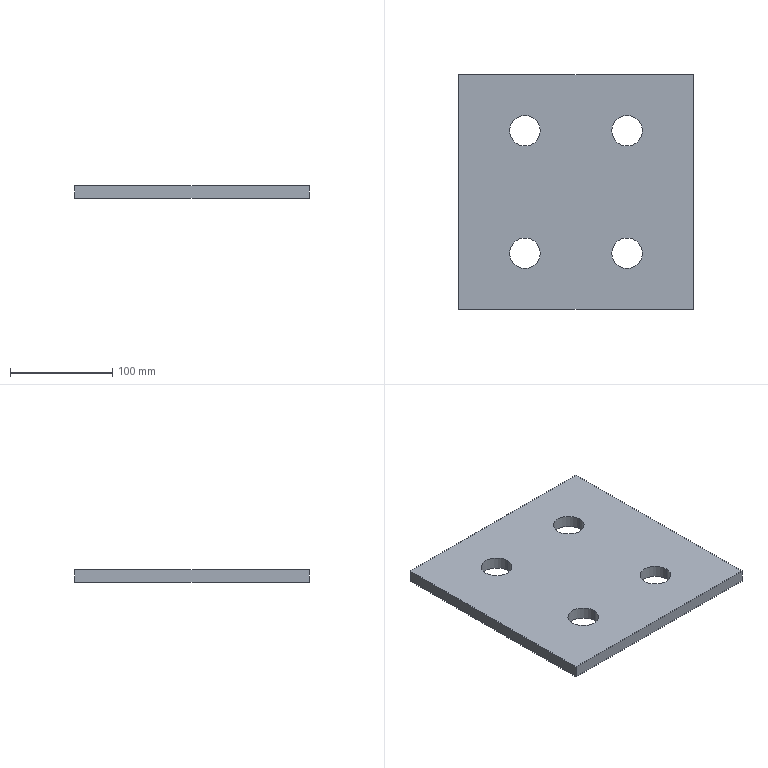Part | STEP file | Reinforcing plate 4 | 1 solid | 14 faces | box 230 x 230 x 12 mm | volume 600871 mm3 | cylinder 8 | plane 6 | commonest cylinder face diameters 30 x8
STEP:
#1=CARTESIAN_POINT('',(0.,0.,0.));
#2=DIRECTION('',(0.,0.,1.));
#3=DIRECTION('',(1.,0.,0.));
#4=AXIS2_PLACEMENT_3D('',#1,#2,#3);
#5=CARTESIAN_POINT('',(35.,-45.,12.));
#6=VERTEX_POINT('',#5);
#7=CARTESIAN_POINT('',(35.,-45.,0.));
#8=VERTEX_POINT('',#7);
#9=CARTESIAN_POINT('',(35.,-45.,12.));
#10=DIRECTION('',(0.,0.,-1.));
#11=VECTOR('',#10,1.);
#12=LINE('',#9,#11);
#13=CARTESIAN_POINT('',(50.,-45.,12.));
#14=DIRECTION('',(0.,0.,-1.));
#15=DIRECTION('',(-1.,0.,0.));
#16=AXIS2_PLACEMENT_3D('',#13,#14,#15);
#17=CYLINDRICAL_SURFACE('',#16,15.);
#18=CARTESIAN_POINT('',(6.283,0.));
#19=DIRECTION('',(0.,1.));
#20=VECTOR('',#19,1.);
#21=LINE('',#18,#20);
#22=(GEOMETRIC_REPRESENTATION_CONTEXT(2)PARAMETRIC_REPRESENTATION_CONTEXT()REPRESENTATION_CONTEXT('',''));
#23=DEFINITIONAL_REPRESENTATION('',(#21),#22);
#24=PCURVE('',#17,#23);
#25=CARTESIAN_POINT('',(50.,-45.,12.));
#26=DIRECTION('',(0.,0.,-1.));
#27=DIRECTION('',(-1.,0.,0.));
#28=AXIS2_PLACEMENT_3D('',#25,#26,#27);
#29=CYLINDRICAL_SURFACE('',#28,15.);
#30=CARTESIAN_POINT('',(0.,0.));
#31=DIRECTION('',(0.,1.));
#32=VECTOR('',#31,1.);
#33=LINE('',#30,#32);
#34=(GEOMETRIC_REPRESENTATION_CONTEXT(2)PARAMETRIC_REPRESENTATION_CONTEXT()REPRESENTATION_CONTEXT('',''));
#35=DEFINITIONAL_REPRESENTATION('',(#33),#34);
#36=PCURVE('',#29,#35);
#37=SURFACE_CURVE('',#12,(#24,#36),.PCURVE_S1.);
#38=EDGE_CURVE('',#6,#8,#37,.T.);
#39=ORIENTED_EDGE('',*,*,#38,.T.);
#40=CARTESIAN_POINT('',(65.,-45.,0.));
#41=VERTEX_POINT('',#40);
#42=CARTESIAN_POINT('',(50.,-45.,0.));
#43=DIRECTION('',(0.,0.,1.));
#44=DIRECTION('',(1.,0.,0.));
#45=AXIS2_PLACEMENT_3D('',#42,#43,#44);
#46=CIRCLE('',#45,15.);
#47=CARTESIAN_POINT('',(9.425,12.));
#48=DIRECTION('',(-1.,0.));
#49=VECTOR('',#48,1.);
#50=LINE('',#47,#49);
#51=(GEOMETRIC_REPRESENTATION_CONTEXT(2)PARAMETRIC_REPRESENTATION_CONTEXT()REPRESENTATION_CONTEXT('',''));
#52=DEFINITIONAL_REPRESENTATION('',(#50),#51);
#53=PCURVE('',#17,#52);
#54=CARTESIAN_POINT('',(115.,-100.,0.));
#55=DIRECTION('',(0.,0.,1.));
#56=DIRECTION('',(1.,0.,0.));
#57=AXIS2_PLACEMENT_3D('',#54,#55,#56);
#58=PLANE('',#57);
#59=CARTESIAN_POINT('',(-65.,55.));
#60=DIRECTION('',(1.,0.));
#61=AXIS2_PLACEMENT_2D('',#59,#60);
#62=CIRCLE('',#61,15.);
#63=(GEOMETRIC_REPRESENTATION_CONTEXT(2)PARAMETRIC_REPRESENTATION_CONTEXT()REPRESENTATION_CONTEXT('',''));
#64=DEFINITIONAL_REPRESENTATION('',(#62),#63);
#65=PCURVE('',#58,#64);
#66=SURFACE_CURVE('',#46,(#53,#65),.PCURVE_S1.);
#67=EDGE_CURVE('',#8,#41,#66,.T.);
#68=ORIENTED_EDGE('',*,*,#67,.T.);
#69=CARTESIAN_POINT('',(65.,-45.,12.));
#70=VERTEX_POINT('',#69);
#71=CARTESIAN_POINT('',(65.,-45.,12.));
#72=DIRECTION('',(0.,0.,-1.));
#73=VECTOR('',#72,1.);
#74=LINE('',#71,#73);
#75=CARTESIAN_POINT('',(3.142,0.));
#76=DIRECTION('',(0.,1.));
#77=VECTOR('',#76,1.);
#78=LINE('',#75,#77);
#79=(GEOMETRIC_REPRESENTATION_CONTEXT(2)PARAMETRIC_REPRESENTATION_CONTEXT()REPRESENTATION_CONTEXT('',''));
#80=DEFINITIONAL_REPRESENTATION('',(#78),#79);
#81=PCURVE('',#17,#80);
#82=CARTESIAN_POINT('',(3.142,0.));
#83=DIRECTION('',(0.,1.));
#84=VECTOR('',#83,1.);
#85=LINE('',#82,#84);
#86=(GEOMETRIC_REPRESENTATION_CONTEXT(2)PARAMETRIC_REPRESENTATION_CONTEXT()REPRESENTATION_CONTEXT('',''));
#87=DEFINITIONAL_REPRESENTATION('',(#85),#86);
#88=PCURVE('',#29,#87);
#89=SURFACE_CURVE('',#74,(#81,#88),.PCURVE_S1.);
#90=EDGE_CURVE('',#70,#41,#89,.T.);
#91=ORIENTED_EDGE('',*,*,#90,.F.);
#92=CARTESIAN_POINT('',(50.,-45.,12.));
#93=DIRECTION('',(0.,0.,1.));
#94=DIRECTION('',(1.,0.,0.));
#95=AXIS2_PLACEMENT_3D('',#92,#93,#94);
#96=CIRCLE('',#95,15.);
#97=CARTESIAN_POINT('',(9.425,0.));
#98=DIRECTION('',(-1.,0.));
#99=VECTOR('',#98,1.);
#100=LINE('',#97,#99);
#101=(GEOMETRIC_REPRESENTATION_CONTEXT(2)PARAMETRIC_REPRESENTATION_CONTEXT()REPRESENTATION_CONTEXT('',''));
#102=DEFINITIONAL_REPRESENTATION('',(#100),#101);
#103=PCURVE('',#17,#102);
#104=CARTESIAN_POINT('',(115.,-100.,12.));
#105=DIRECTION('',(0.,0.,1.));
#106=DIRECTION('',(1.,0.,0.));
#107=AXIS2_PLACEMENT_3D('',#104,#105,#106);
#108=PLANE('',#107);
#109=CARTESIAN_POINT('',(-65.,55.));
#110=DIRECTION('',(1.,0.));
#111=AXIS2_PLACEMENT_2D('',#109,#110);
#112=CIRCLE('',#111,15.);
#113=(GEOMETRIC_REPRESENTATION_CONTEXT(2)PARAMETRIC_REPRESENTATION_CONTEXT()REPRESENTATION_CONTEXT('',''));
#114=DEFINITIONAL_REPRESENTATION('',(#112),#113);
#115=PCURVE('',#108,#114);
#116=SURFACE_CURVE('',#96,(#103,#115),.PCURVE_S1.);
#117=EDGE_CURVE('',#6,#70,#116,.T.);
#118=ORIENTED_EDGE('',*,*,#117,.F.);
#119=EDGE_LOOP('',(#39,#68,#91,#118));
#120=FACE_BOUND('',#119,.F.);
#121=ADVANCED_FACE('',(#120),#17,.F.);
#122=CARTESIAN_POINT('',(-65.,-45.,12.));
#123=VERTEX_POINT('',#122);
#124=CARTESIAN_POINT('',(-65.,-45.,0.));
#125=VERTEX_POINT('',#124);
#126=CARTESIAN_POINT('',(-65.,-45.,12.));
#127=DIRECTION('',(0.,0.,-1.));
#128=VECTOR('',#127,1.);
#129=LINE('',#126,#128);
#130=CARTESIAN_POINT('',(-50.,-45.,12.));
#131=DIRECTION('',(0.,0.,-1.));
#132=DIRECTION('',(-1.,0.,0.));
#133=AXIS2_PLACEMENT_3D('',#130,#131,#132);
#134=CYLINDRICAL_SURFACE('',#133,15.);
#135=CARTESIAN_POINT('',(6.283,0.));
#136=DIRECTION('',(0.,1.));
#137=VECTOR('',#136,1.);
#138=LINE('',#135,#137);
#139=(GEOMETRIC_REPRESENTATION_CONTEXT(2)PARAMETRIC_REPRESENTATION_CONTEXT()REPRESENTATION_CONTEXT('',''));
#140=DEFINITIONAL_REPRESENTATION('',(#138),#139);
#141=PCURVE('',#134,#140);
#142=CARTESIAN_POINT('',(-50.,-45.,12.));
#143=DIRECTION('',(0.,0.,-1.));
#144=DIRECTION('',(-1.,0.,0.));
#145=AXIS2_PLACEMENT_3D('',#142,#143,#144);
#146=CYLINDRICAL_SURFACE('',#145,15.);
#147=CARTESIAN_POINT('',(0.,0.));
#148=DIRECTION('',(0.,1.));
#149=VECTOR('',#148,1.);
#150=LINE('',#147,#149);
#151=(GEOMETRIC_REPRESENTATION_CONTEXT(2)PARAMETRIC_REPRESENTATION_CONTEXT()REPRESENTATION_CONTEXT('',''));
#152=DEFINITIONAL_REPRESENTATION('',(#150),#151);
#153=PCURVE('',#146,#152);
#154=SURFACE_CURVE('',#129,(#141,#153),.PCURVE_S1.);
#155=EDGE_CURVE('',#123,#125,#154,.T.);
#156=ORIENTED_EDGE('',*,*,#155,.T.);
#157=CARTESIAN_POINT('',(-35.,-45.,0.));
#158=VERTEX_POINT('',#157);
#159=CARTESIAN_POINT('',(-50.,-45.,0.));
#160=DIRECTION('',(0.,0.,1.));
#161=DIRECTION('',(1.,0.,0.));
#162=AXIS2_PLACEMENT_3D('',#159,#160,#161);
#163=CIRCLE('',#162,15.);
#164=CARTESIAN_POINT('',(9.425,12.));
#165=DIRECTION('',(-1.,0.));
#166=VECTOR('',#165,1.);
#167=LINE('',#164,#166);
#168=(GEOMETRIC_REPRESENTATION_CONTEXT(2)PARAMETRIC_REPRESENTATION_CONTEXT()REPRESENTATION_CONTEXT('',''));
#169=DEFINITIONAL_REPRESENTATION('',(#167),#168);
#170=PCURVE('',#134,#169);
#171=CARTESIAN_POINT('',(-165.,55.));
#172=DIRECTION('',(1.,0.));
#173=AXIS2_PLACEMENT_2D('',#171,#172);
#174=CIRCLE('',#173,15.);
#175=(GEOMETRIC_REPRESENTATION_CONTEXT(2)PARAMETRIC_REPRESENTATION_CONTEXT()REPRESENTATION_CONTEXT('',''));
#176=DEFINITIONAL_REPRESENTATION('',(#174),#175);
#177=PCURVE('',#58,#176);
#178=SURFACE_CURVE('',#163,(#170,#177),.PCURVE_S1.);
#179=EDGE_CURVE('',#125,#158,#178,.T.);
#180=ORIENTED_EDGE('',*,*,#179,.T.);
#181=CARTESIAN_POINT('',(-35.,-45.,12.));
#182=VERTEX_POINT('',#181);
#183=CARTESIAN_POINT('',(-35.,-45.,12.));
#184=DIRECTION('',(0.,0.,-1.));
#185=VECTOR('',#184,1.);
#186=LINE('',#183,#185);
#187=CARTESIAN_POINT('',(3.142,0.));
#188=DIRECTION('',(0.,1.));
#189=VECTOR('',#188,1.);
#190=LINE('',#187,#189);
#191=(GEOMETRIC_REPRESENTATION_CONTEXT(2)PARAMETRIC_REPRESENTATION_CONTEXT()REPRESENTATION_CONTEXT('',''));
#192=DEFINITIONAL_REPRESENTATION('',(#190),#191);
#193=PCURVE('',#134,#192);
#194=CARTESIAN_POINT('',(3.142,0.));
#195=DIRECTION('',(0.,1.));
#196=VECTOR('',#195,1.);
#197=LINE('',#194,#196);
#198=(GEOMETRIC_REPRESENTATION_CONTEXT(2)PARAMETRIC_REPRESENTATION_CONTEXT()REPRESENTATION_CONTEXT('',''));
#199=DEFINITIONAL_REPRESENTATION('',(#197),#198);
#200=PCURVE('',#146,#199);
#201=SURFACE_CURVE('',#186,(#193,#200),.PCURVE_S1.);
#202=EDGE_CURVE('',#182,#158,#201,.T.);
#203=ORIENTED_EDGE('',*,*,#202,.F.);
#204=CARTESIAN_POINT('',(-50.,-45.,12.));
#205=DIRECTION('',(0.,0.,1.));
#206=DIRECTION('',(1.,0.,0.));
#207=AXIS2_PLACEMENT_3D('',#204,#205,#206);
#208=CIRCLE('',#207,15.);
#209=CARTESIAN_POINT('',(9.425,0.));
#210=DIRECTION('',(-1.,0.));
#211=VECTOR('',#210,1.);
#212=LINE('',#209,#211);
#213=(GEOMETRIC_REPRESENTATION_CONTEXT(2)PARAMETRIC_REPRESENTATION_CONTEXT()REPRESENTATION_CONTEXT('',''));
#214=DEFINITIONAL_REPRESENTATION('',(#212),#213);
#215=PCURVE('',#134,#214);
#216=CARTESIAN_POINT('',(-165.,55.));
#217=DIRECTION('',(1.,0.));
#218=AXIS2_PLACEMENT_2D('',#216,#217);
#219=CIRCLE('',#218,15.);
#220=(GEOMETRIC_REPRESENTATION_CONTEXT(2)PARAMETRIC_REPRESENTATION_CONTEXT()REPRESENTATION_CONTEXT('',''));
#221=DEFINITIONAL_REPRESENTATION('',(#219),#220);
#222=PCURVE('',#108,#221);
#223=SURFACE_CURVE('',#208,(#215,#222),.PCURVE_S1.);
#224=EDGE_CURVE('',#123,#182,#223,.T.);
#225=ORIENTED_EDGE('',*,*,#224,.F.);
#226=EDGE_LOOP('',(#156,#180,#203,#225));
#227=FACE_BOUND('',#226,.F.);
#228=ADVANCED_FACE('',(#227),#134,.F.);
#229=CARTESIAN_POINT('',(35.,75.,12.));
#230=VERTEX_POINT('',#229);
#231=CARTESIAN_POINT('',(35.,75.,0.));
#232=VERTEX_POINT('',#231);
#233=CARTESIAN_POINT('',(35.,75.,12.));
#234=DIRECTION('',(0.,0.,-1.));
#235=VECTOR('',#234,1.);
#236=LINE('',#233,#235);
#237=CARTESIAN_POINT('',(50.,75.,12.));
#238=DIRECTION('',(0.,0.,-1.));
#239=DIRECTION('',(-1.,0.,0.));
#240=AXIS2_PLACEMENT_3D('',#237,#238,#239);
#241=CYLINDRICAL_SURFACE('',#240,15.);
#242=CARTESIAN_POINT('',(6.283,0.));
#243=DIRECTION('',(0.,1.));
#244=VECTOR('',#243,1.);
#245=LINE('',#242,#244);
#246=(GEOMETRIC_REPRESENTATION_CONTEXT(2)PARAMETRIC_REPRESENTATION_CONTEXT()REPRESENTATION_CONTEXT('',''));
#247=DEFINITIONAL_REPRESENTATION('',(#245),#246);
#248=PCURVE('',#241,#247);
#249=CARTESIAN_POINT('',(50.,75.,12.));
#250=DIRECTION('',(0.,0.,-1.));
#251=DIRECTION('',(-1.,0.,0.));
#252=AXIS2_PLACEMENT_3D('',#249,#250,#251);
#253=CYLINDRICAL_SURFACE('',#252,15.);
#254=CARTESIAN_POINT('',(0.,0.));
#255=DIRECTION('',(0.,1.));
#256=VECTOR('',#255,1.);
#257=LINE('',#254,#256);
#258=(GEOMETRIC_REPRESENTATION_CONTEXT(2)PARAMETRIC_REPRESENTATION_CONTEXT()REPRESENTATION_CONTEXT('',''));
#259=DEFINITIONAL_REPRESENTATION('',(#257),#258);
#260=PCURVE('',#253,#259);
#261=SURFACE_CURVE('',#236,(#248,#260),.PCURVE_S1.);
#262=EDGE_CURVE('',#230,#232,#261,.T.);
#263=ORIENTED_EDGE('',*,*,#262,.T.);
#264=CARTESIAN_POINT('',(65.,75.,0.));
#265=VERTEX_POINT('',#264);
#266=CARTESIAN_POINT('',(50.,75.,0.));
#267=DIRECTION('',(0.,0.,1.));
#268=DIRECTION('',(1.,0.,0.));
#269=AXIS2_PLACEMENT_3D('',#266,#267,#268);
#270=CIRCLE('',#269,15.);
#271=CARTESIAN_POINT('',(9.425,12.));
#272=DIRECTION('',(-1.,0.));
#273=VECTOR('',#272,1.);
#274=LINE('',#271,#273);
#275=(GEOMETRIC_REPRESENTATION_CONTEXT(2)PARAMETRIC_REPRESENTATION_CONTEXT()REPRESENTATION_CONTEXT('',''));
#276=DEFINITIONAL_REPRESENTATION('',(#274),#275);
#277=PCURVE('',#241,#276);
#278=CARTESIAN_POINT('',(-65.,175.));
#279=DIRECTION('',(1.,0.));
#280=AXIS2_PLACEMENT_2D('',#278,#279);
#281=CIRCLE('',#280,15.);
#282=(GEOMETRIC_REPRESENTATION_CONTEXT(2)PARAMETRIC_REPRESENTATION_CONTEXT()REPRESENTATION_CONTEXT('',''));
#283=DEFINITIONAL_REPRESENTATION('',(#281),#282);
#284=PCURVE('',#58,#283);
#285=SURFACE_CURVE('',#270,(#277,#284),.PCURVE_S1.);
#286=EDGE_CURVE('',#232,#265,#285,.T.);
#287=ORIENTED_EDGE('',*,*,#286,.T.);
#288=CARTESIAN_POINT('',(65.,75.,12.));
#289=VERTEX_POINT('',#288);
#290=CARTESIAN_POINT('',(65.,75.,12.));
#291=DIRECTION('',(0.,0.,-1.));
#292=VECTOR('',#291,1.);
#293=LINE('',#290,#292);
#294=CARTESIAN_POINT('',(3.142,0.));
#295=DIRECTION('',(0.,1.));
#296=VECTOR('',#295,1.);
#297=LINE('',#294,#296);
#298=(GEOMETRIC_REPRESENTATION_CONTEXT(2)PARAMETRIC_REPRESENTATION_CONTEXT()REPRESENTATION_CONTEXT('',''));
#299=DEFINITIONAL_REPRESENTATION('',(#297),#298);
#300=PCURVE('',#241,#299);
#301=CARTESIAN_POINT('',(3.142,0.));
#302=DIRECTION('',(0.,1.));
#303=VECTOR('',#302,1.);
#304=LINE('',#301,#303);
#305=(GEOMETRIC_REPRESENTATION_CONTEXT(2)PARAMETRIC_REPRESENTATION_CONTEXT()REPRESENTATION_CONTEXT('',''));
#306=DEFINITIONAL_REPRESENTATION('',(#304),#305);
#307=PCURVE('',#253,#306);
#308=SURFACE_CURVE('',#293,(#300,#307),.PCURVE_S1.);
#309=EDGE_CURVE('',#289,#265,#308,.T.);
#310=ORIENTED_EDGE('',*,*,#309,.F.);
#311=CARTESIAN_POINT('',(50.,75.,12.));
#312=DIRECTION('',(0.,0.,1.));
#313=DIRECTION('',(1.,0.,0.));
#314=AXIS2_PLACEMENT_3D('',#311,#312,#313);
#315=CIRCLE('',#314,15.);
#316=CARTESIAN_POINT('',(9.425,0.));
#317=DIRECTION('',(-1.,0.));
#318=VECTOR('',#317,1.);
#319=LINE('',#316,#318);
#320=(GEOMETRIC_REPRESENTATION_CONTEXT(2)PARAMETRIC_REPRESENTATION_CONTEXT()REPRESENTATION_CONTEXT('',''));
#321=DEFINITIONAL_REPRESENTATION('',(#319),#320);
#322=PCURVE('',#241,#321);
#323=CARTESIAN_POINT('',(-65.,175.));
#324=DIRECTION('',(1.,0.));
#325=AXIS2_PLACEMENT_2D('',#323,#324);
#326=CIRCLE('',#325,15.);
#327=(GEOMETRIC_REPRESENTATION_CONTEXT(2)PARAMETRIC_REPRESENTATION_CONTEXT()REPRESENTATION_CONTEXT('',''));
#328=DEFINITIONAL_REPRESENTATION('',(#326),#327);
#329=PCURVE('',#108,#328);
#330=SURFACE_CURVE('',#315,(#322,#329),.PCURVE_S1.);
#331=EDGE_CURVE('',#230,#289,#330,.T.);
#332=ORIENTED_EDGE('',*,*,#331,.F.);
#333=EDGE_LOOP('',(#263,#287,#310,#332));
#334=FACE_BOUND('',#333,.F.);
#335=ADVANCED_FACE('',(#334),#241,.F.);
#336=CARTESIAN_POINT('',(-65.,75.,12.));
#337=VERTEX_POINT('',#336);
#338=CARTESIAN_POINT('',(-65.,75.,0.));
#339=VERTEX_POINT('',#338);
#340=CARTESIAN_POINT('',(-65.,75.,12.));
#341=DIRECTION('',(0.,0.,-1.));
#342=VECTOR('',#341,1.);
#343=LINE('',#340,#342);
#344=CARTESIAN_POINT('',(-50.,75.,12.));
#345=DIRECTION('',(0.,0.,-1.));
#346=DIRECTION('',(-1.,0.,0.));
#347=AXIS2_PLACEMENT_3D('',#344,#345,#346);
#348=CYLINDRICAL_SURFACE('',#347,15.);
#349=CARTESIAN_POINT('',(6.283,0.));
#350=DIRECTION('',(0.,1.));
#351=VECTOR('',#350,1.);
#352=LINE('',#349,#351);
#353=(GEOMETRIC_REPRESENTATION_CONTEXT(2)PARAMETRIC_REPRESENTATION_CONTEXT()REPRESENTATION_CONTEXT('',''));
#354=DEFINITIONAL_REPRESENTATION('',(#352),#353);
#355=PCURVE('',#348,#354);
#356=CARTESIAN_POINT('',(-50.,75.,12.));
#357=DIRECTION('',(0.,0.,-1.));
#358=DIRECTION('',(-1.,0.,0.));
#359=AXIS2_PLACEMENT_3D('',#356,#357,#358);
#360=CYLINDRICAL_SURFACE('',#359,15.);
#361=CARTESIAN_POINT('',(0.,0.));
#362=DIRECTION('',(0.,1.));
#363=VECTOR('',#362,1.);
#364=LINE('',#361,#363);
#365=(GEOMETRIC_REPRESENTATION_CONTEXT(2)PARAMETRIC_REPRESENTATION_CONTEXT()REPRESENTATION_CONTEXT('',''));
#366=DEFINITIONAL_REPRESENTATION('',(#364),#365);
#367=PCURVE('',#360,#366);
#368=SURFACE_CURVE('',#343,(#355,#367),.PCURVE_S1.);
#369=EDGE_CURVE('',#337,#339,#368,.T.);
#370=ORIENTED_EDGE('',*,*,#369,.T.);
#371=CARTESIAN_POINT('',(-35.,75.,0.));
#372=VERTEX_POINT('',#371);
#373=CARTESIAN_POINT('',(-50.,75.,0.));
#374=DIRECTION('',(0.,0.,1.));
#375=DIRECTION('',(1.,0.,0.));
#376=AXIS2_PLACEMENT_3D('',#373,#374,#375);
#377=CIRCLE('',#376,15.);
#378=CARTESIAN_POINT('',(9.425,12.));
#379=DIRECTION('',(-1.,0.));
#380=VECTOR('',#379,1.);
#381=LINE('',#378,#380);
#382=(GEOMETRIC_REPRESENTATION_CONTEXT(2)PARAMETRIC_REPRESENTATION_CONTEXT()REPRESENTATION_CONTEXT('',''));
#383=DEFINITIONAL_REPRESENTATION('',(#381),#382);
#384=PCURVE('',#348,#383);
#385=CARTESIAN_POINT('',(-165.,175.));
#386=DIRECTION('',(1.,0.));
#387=AXIS2_PLACEMENT_2D('',#385,#386);
#388=CIRCLE('',#387,15.);
#389=(GEOMETRIC_REPRESENTATION_CONTEXT(2)PARAMETRIC_REPRESENTATION_CONTEXT()REPRESENTATION_CONTEXT('',''));
#390=DEFINITIONAL_REPRESENTATION('',(#388),#389);
#391=PCURVE('',#58,#390);
#392=SURFACE_CURVE('',#377,(#384,#391),.PCURVE_S1.);
#393=EDGE_CURVE('',#339,#372,#392,.T.);
#394=ORIENTED_EDGE('',*,*,#393,.T.);
#395=CARTESIAN_POINT('',(-35.,75.,12.));
#396=VERTEX_POINT('',#395);
#397=CARTESIAN_POINT('',(-35.,75.,12.));
#398=DIRECTION('',(0.,0.,-1.));
#399=VECTOR('',#398,1.);
#400=LINE('',#397,#399);
#401=CARTESIAN_POINT('',(3.142,0.));
#402=DIRECTION('',(0.,1.));
#403=VECTOR('',#402,1.);
#404=LINE('',#401,#403);
#405=(GEOMETRIC_REPRESENTATION_CONTEXT(2)PARAMETRIC_REPRESENTATION_CONTEXT()REPRESENTATION_CONTEXT('',''));
#406=DEFINITIONAL_REPRESENTATION('',(#404),#405);
#407=PCURVE('',#348,#406);
#408=CARTESIAN_POINT('',(3.142,0.));
#409=DIRECTION('',(0.,1.));
#410=VECTOR('',#409,1.);
#411=LINE('',#408,#410);
#412=(GEOMETRIC_REPRESENTATION_CONTEXT(2)PARAMETRIC_REPRESENTATION_CONTEXT()REPRESENTATION_CONTEXT('',''));
#413=DEFINITIONAL_REPRESENTATION('',(#411),#412);
#414=PCURVE('',#360,#413);
#415=SURFACE_CURVE('',#400,(#407,#414),.PCURVE_S1.);
#416=EDGE_CURVE('',#396,#372,#415,.T.);
#417=ORIENTED_EDGE('',*,*,#416,.F.);
#418=CARTESIAN_POINT('',(-50.,75.,12.));
#419=DIRECTION('',(0.,0.,1.));
#420=DIRECTION('',(1.,0.,0.));
#421=AXIS2_PLACEMENT_3D('',#418,#419,#420);
#422=CIRCLE('',#421,15.);
#423=CARTESIAN_POINT('',(9.425,0.));
#424=DIRECTION('',(-1.,0.));
#425=VECTOR('',#424,1.);
#426=LINE('',#423,#425);
#427=(GEOMETRIC_REPRESENTATION_CONTEXT(2)PARAMETRIC_REPRESENTATION_CONTEXT()REPRESENTATION_CONTEXT('',''));
#428=DEFINITIONAL_REPRESENTATION('',(#426),#427);
#429=PCURVE('',#348,#428);
#430=CARTESIAN_POINT('',(-165.,175.));
#431=DIRECTION('',(1.,0.));
#432=AXIS2_PLACEMENT_2D('',#430,#431);
#433=CIRCLE('',#432,15.);
#434=(GEOMETRIC_REPRESENTATION_CONTEXT(2)PARAMETRIC_REPRESENTATION_CONTEXT()REPRESENTATION_CONTEXT('',''));
#435=DEFINITIONAL_REPRESENTATION('',(#433),#434);
#436=PCURVE('',#108,#435);
#437=SURFACE_CURVE('',#422,(#429,#436),.PCURVE_S1.);
#438=EDGE_CURVE('',#337,#396,#437,.T.);
#439=ORIENTED_EDGE('',*,*,#438,.F.);
#440=EDGE_LOOP('',(#370,#394,#417,#439));
#441=FACE_BOUND('',#440,.F.);
#442=ADVANCED_FACE('',(#441),#348,.F.);
#443=ORIENTED_EDGE('',*,*,#224,.F.);
#444=CARTESIAN_POINT('',(-50.,-45.,12.));
#445=DIRECTION('',(0.,0.,1.));
#446=DIRECTION('',(1.,0.,0.));
#447=AXIS2_PLACEMENT_3D('',#444,#445,#446);
#448=CIRCLE('',#447,15.);
#449=CARTESIAN_POINT('',(-165.,55.));
#450=DIRECTION('',(1.,0.));
#451=AXIS2_PLACEMENT_2D('',#449,#450);
#452=CIRCLE('',#451,15.);
#453=(GEOMETRIC_REPRESENTATION_CONTEXT(2)PARAMETRIC_REPRESENTATION_CONTEXT()REPRESENTATION_CONTEXT('',''));
#454=DEFINITIONAL_REPRESENTATION('',(#452),#453);
#455=PCURVE('',#108,#454);
#456=CARTESIAN_POINT('',(3.142,0.));
#457=DIRECTION('',(-1.,0.));
#458=VECTOR('',#457,1.);
#459=LINE('',#456,#458);
#460=(GEOMETRIC_REPRESENTATION_CONTEXT(2)PARAMETRIC_REPRESENTATION_CONTEXT()REPRESENTATION_CONTEXT('',''));
#461=DEFINITIONAL_REPRESENTATION('',(#459),#460);
#462=PCURVE('',#146,#461);
#463=SURFACE_CURVE('',#448,(#455,#462),.PCURVE_S1.);
#464=EDGE_CURVE('',#182,#123,#463,.T.);
#465=ORIENTED_EDGE('',*,*,#464,.F.);
#466=EDGE_LOOP('',(#443,#465));
#467=FACE_BOUND('',#466,.T.);
#468=ORIENTED_EDGE('',*,*,#438,.F.);
#469=CARTESIAN_POINT('',(-50.,75.,12.));
#470=DIRECTION('',(0.,0.,1.));
#471=DIRECTION('',(1.,0.,0.));
#472=AXIS2_PLACEMENT_3D('',#469,#470,#471);
#473=CIRCLE('',#472,15.);
#474=CARTESIAN_POINT('',(-165.,175.));
#475=DIRECTION('',(1.,0.));
#476=AXIS2_PLACEMENT_2D('',#474,#475);
#477=CIRCLE('',#476,15.);
#478=(GEOMETRIC_REPRESENTATION_CONTEXT(2)PARAMETRIC_REPRESENTATION_CONTEXT()REPRESENTATION_CONTEXT('',''));
#479=DEFINITIONAL_REPRESENTATION('',(#477),#478);
#480=PCURVE('',#108,#479);
#481=CARTESIAN_POINT('',(3.142,0.));
#482=DIRECTION('',(-1.,0.));
#483=VECTOR('',#482,1.);
#484=LINE('',#481,#483);
#485=(GEOMETRIC_REPRESENTATION_CONTEXT(2)PARAMETRIC_REPRESENTATION_CONTEXT()REPRESENTATION_CONTEXT('',''));
#486=DEFINITIONAL_REPRESENTATION('',(#484),#485);
#487=PCURVE('',#360,#486);
#488=SURFACE_CURVE('',#473,(#480,#487),.PCURVE_S1.);
#489=EDGE_CURVE('',#396,#337,#488,.T.);
#490=ORIENTED_EDGE('',*,*,#489,.F.);
#491=EDGE_LOOP('',(#468,#490));
#492=FACE_BOUND('',#491,.T.);
#493=CARTESIAN_POINT('',(115.,-100.,12.));
#494=VERTEX_POINT('',#493);
#495=CARTESIAN_POINT('',(115.,130.,12.));
#496=VERTEX_POINT('',#495);
#497=CARTESIAN_POINT('',(115.,130.,12.));
#498=DIRECTION('',(0.,1.,0.));
#499=VECTOR('',#498,1.);
#500=LINE('',#497,#499);
#501=CARTESIAN_POINT('',(0.,230.));
#502=DIRECTION('',(0.,1.));
#503=VECTOR('',#502,1.);
#504=LINE('',#501,#503);
#505=(GEOMETRIC_REPRESENTATION_CONTEXT(2)PARAMETRIC_REPRESENTATION_CONTEXT()REPRESENTATION_CONTEXT('',''));
#506=DEFINITIONAL_REPRESENTATION('',(#504),#505);
#507=PCURVE('',#108,#506);
#508=CARTESIAN_POINT('',(115.,130.,12.));
#509=DIRECTION('',(-1.,0.,0.));
#510=DIRECTION('',(0.,-1.,0.));
#511=AXIS2_PLACEMENT_3D('',#508,#509,#510);
#512=PLANE('',#511);
#513=CARTESIAN_POINT('',(0.,0.));
#514=DIRECTION('',(-1.,0.));
#515=VECTOR('',#514,1.);
#516=LINE('',#513,#515);
#517=(GEOMETRIC_REPRESENTATION_CONTEXT(2)PARAMETRIC_REPRESENTATION_CONTEXT()REPRESENTATION_CONTEXT('',''));
#518=DEFINITIONAL_REPRESENTATION('',(#516),#517);
#519=PCURVE('',#512,#518);
#520=SURFACE_CURVE('',#500,(#507,#519),.PCURVE_S1.);
#521=EDGE_CURVE('',#494,#496,#520,.T.);
#522=ORIENTED_EDGE('',*,*,#521,.T.);
#523=CARTESIAN_POINT('',(-115.,130.,12.));
#524=VERTEX_POINT('',#523);
#525=CARTESIAN_POINT('',(-115.,130.,12.));
#526=DIRECTION('',(-1.,0.,0.));
#527=VECTOR('',#526,1.);
#528=LINE('',#525,#527);
#529=CARTESIAN_POINT('',(-230.,230.));
#530=DIRECTION('',(-1.,0.));
#531=VECTOR('',#530,1.);
#532=LINE('',#529,#531);
#533=(GEOMETRIC_REPRESENTATION_CONTEXT(2)PARAMETRIC_REPRESENTATION_CONTEXT()REPRESENTATION_CONTEXT('',''));
#534=DEFINITIONAL_REPRESENTATION('',(#532),#533);
#535=PCURVE('',#108,#534);
#536=CARTESIAN_POINT('',(-115.,130.,12.));
#537=DIRECTION('',(0.,-1.,0.));
#538=DIRECTION('',(0.,0.,-1.));
#539=AXIS2_PLACEMENT_3D('',#536,#537,#538);
#540=PLANE('',#539);
#541=CARTESIAN_POINT('',(0.,0.));
#542=DIRECTION('',(0.,-1.));
#543=VECTOR('',#542,1.);
#544=LINE('',#541,#543);
#545=(GEOMETRIC_REPRESENTATION_CONTEXT(2)PARAMETRIC_REPRESENTATION_CONTEXT()REPRESENTATION_CONTEXT('',''));
#546=DEFINITIONAL_REPRESENTATION('',(#544),#545);
#547=PCURVE('',#540,#546);
#548=SURFACE_CURVE('',#528,(#535,#547),.PCURVE_S1.);
#549=EDGE_CURVE('',#496,#524,#548,.T.);
#550=ORIENTED_EDGE('',*,*,#549,.T.);
#551=CARTESIAN_POINT('',(-115.,-100.,12.));
#552=VERTEX_POINT('',#551);
#553=CARTESIAN_POINT('',(-115.,130.,12.));
#554=DIRECTION('',(0.,-1.,0.));
#555=VECTOR('',#554,1.);
#556=LINE('',#553,#555);
#557=CARTESIAN_POINT('',(-230.,230.));
#558=DIRECTION('',(0.,-1.));
#559=VECTOR('',#558,1.);
#560=LINE('',#557,#559);
#561=(GEOMETRIC_REPRESENTATION_CONTEXT(2)PARAMETRIC_REPRESENTATION_CONTEXT()REPRESENTATION_CONTEXT('',''));
#562=DEFINITIONAL_REPRESENTATION('',(#560),#561);
#563=PCURVE('',#108,#562);
#564=CARTESIAN_POINT('',(-115.,130.,12.));
#565=DIRECTION('',(1.,0.,0.));
#566=DIRECTION('',(0.,1.,0.));
#567=AXIS2_PLACEMENT_3D('',#564,#565,#566);
#568=PLANE('',#567);
#569=CARTESIAN_POINT('',(0.,0.));
#570=DIRECTION('',(-1.,0.));
#571=VECTOR('',#570,1.);
#572=LINE('',#569,#571);
#573=(GEOMETRIC_REPRESENTATION_CONTEXT(2)PARAMETRIC_REPRESENTATION_CONTEXT()REPRESENTATION_CONTEXT('',''));
#574=DEFINITIONAL_REPRESENTATION('',(#572),#573);
#575=PCURVE('',#568,#574);
#576=SURFACE_CURVE('',#556,(#563,#575),.PCURVE_S1.);
#577=EDGE_CURVE('',#524,#552,#576,.T.);
#578=ORIENTED_EDGE('',*,*,#577,.T.);
#579=CARTESIAN_POINT('',(-115.,-100.,12.));
#580=DIRECTION('',(1.,0.,0.));
#581=VECTOR('',#580,1.);
#582=LINE('',#579,#581);
#583=CARTESIAN_POINT('',(-230.,0.));
#584=DIRECTION('',(1.,0.));
#585=VECTOR('',#584,1.);
#586=LINE('',#583,#585);
#587=(GEOMETRIC_REPRESENTATION_CONTEXT(2)PARAMETRIC_REPRESENTATION_CONTEXT()REPRESENTATION_CONTEXT('',''));
#588=DEFINITIONAL_REPRESENTATION('',(#586),#587);
#589=PCURVE('',#108,#588);
#590=CARTESIAN_POINT('',(-115.,-100.,12.));
#591=DIRECTION('',(0.,1.,0.));
#592=DIRECTION('',(0.,0.,1.));
#593=AXIS2_PLACEMENT_3D('',#590,#591,#592);
#594=PLANE('',#593);
#595=CARTESIAN_POINT('',(0.,0.));
#596=DIRECTION('',(0.,1.));
#597=VECTOR('',#596,1.);
#598=LINE('',#595,#597);
#599=(GEOMETRIC_REPRESENTATION_CONTEXT(2)PARAMETRIC_REPRESENTATION_CONTEXT()REPRESENTATION_CONTEXT('',''));
#600=DEFINITIONAL_REPRESENTATION('',(#598),#599);
#601=PCURVE('',#594,#600);
#602=SURFACE_CURVE('',#582,(#589,#601),.PCURVE_S1.);
#603=EDGE_CURVE('',#552,#494,#602,.T.);
#604=ORIENTED_EDGE('',*,*,#603,.T.);
#605=EDGE_LOOP('',(#522,#550,#578,#604));
#606=FACE_BOUND('',#605,.T.);
#607=ORIENTED_EDGE('',*,*,#331,.F.);
#608=CARTESIAN_POINT('',(50.,75.,12.));
#609=DIRECTION('',(0.,0.,1.));
#610=DIRECTION('',(1.,0.,0.));
#611=AXIS2_PLACEMENT_3D('',#608,#609,#610);
#612=CIRCLE('',#611,15.);
#613=CARTESIAN_POINT('',(-65.,175.));
#614=DIRECTION('',(1.,0.));
#615=AXIS2_PLACEMENT_2D('',#613,#614);
#616=CIRCLE('',#615,15.);
#617=(GEOMETRIC_REPRESENTATION_CONTEXT(2)PARAMETRIC_REPRESENTATION_CONTEXT()REPRESENTATION_CONTEXT('',''));
#618=DEFINITIONAL_REPRESENTATION('',(#616),#617);
#619=PCURVE('',#108,#618);
#620=CARTESIAN_POINT('',(3.142,0.));
#621=DIRECTION('',(-1.,0.));
#622=VECTOR('',#621,1.);
#623=LINE('',#620,#622);
#624=(GEOMETRIC_REPRESENTATION_CONTEXT(2)PARAMETRIC_REPRESENTATION_CONTEXT()REPRESENTATION_CONTEXT('',''));
#625=DEFINITIONAL_REPRESENTATION('',(#623),#624);
#626=PCURVE('',#253,#625);
#627=SURFACE_CURVE('',#612,(#619,#626),.PCURVE_S1.);
#628=EDGE_CURVE('',#289,#230,#627,.T.);
#629=ORIENTED_EDGE('',*,*,#628,.F.);
#630=EDGE_LOOP('',(#607,#629));
#631=FACE_BOUND('',#630,.T.);
#632=ORIENTED_EDGE('',*,*,#117,.F.);
#633=CARTESIAN_POINT('',(50.,-45.,12.));
#634=DIRECTION('',(0.,0.,1.));
#635=DIRECTION('',(1.,0.,0.));
#636=AXIS2_PLACEMENT_3D('',#633,#634,#635);
#637=CIRCLE('',#636,15.);
#638=CARTESIAN_POINT('',(-65.,55.));
#639=DIRECTION('',(1.,0.));
#640=AXIS2_PLACEMENT_2D('',#638,#639);
#641=CIRCLE('',#640,15.);
#642=(GEOMETRIC_REPRESENTATION_CONTEXT(2)PARAMETRIC_REPRESENTATION_CONTEXT()REPRESENTATION_CONTEXT('',''));
#643=DEFINITIONAL_REPRESENTATION('',(#641),#642);
#644=PCURVE('',#108,#643);
#645=CARTESIAN_POINT('',(3.142,0.));
#646=DIRECTION('',(-1.,0.));
#647=VECTOR('',#646,1.);
#648=LINE('',#645,#647);
#649=(GEOMETRIC_REPRESENTATION_CONTEXT(2)PARAMETRIC_REPRESENTATION_CONTEXT()REPRESENTATION_CONTEXT('',''));
#650=DEFINITIONAL_REPRESENTATION('',(#648),#649);
#651=PCURVE('',#29,#650);
#652=SURFACE_CURVE('',#637,(#644,#651),.PCURVE_S1.);
#653=EDGE_CURVE('',#70,#6,#652,.T.);
#654=ORIENTED_EDGE('',*,*,#653,.F.);
#655=EDGE_LOOP('',(#632,#654));
#656=FACE_BOUND('',#655,.T.);
#657=ADVANCED_FACE('',(#467,#492,#606,#631,#656),#108,.T.);
#658=ORIENTED_EDGE('',*,*,#179,.T.);
#659=CARTESIAN_POINT('',(-50.,-45.,0.));
#660=DIRECTION('',(0.,0.,1.));
#661=DIRECTION('',(1.,0.,0.));
#662=AXIS2_PLACEMENT_3D('',#659,#660,#661);
#663=CIRCLE('',#662,15.);
#664=CARTESIAN_POINT('',(-165.,55.));
#665=DIRECTION('',(1.,0.));
#666=AXIS2_PLACEMENT_2D('',#664,#665);
#667=CIRCLE('',#666,15.);
#668=(GEOMETRIC_REPRESENTATION_CONTEXT(2)PARAMETRIC_REPRESENTATION_CONTEXT()REPRESENTATION_CONTEXT('',''));
#669=DEFINITIONAL_REPRESENTATION('',(#667),#668);
#670=PCURVE('',#58,#669);
#671=CARTESIAN_POINT('',(3.142,12.));
#672=DIRECTION('',(-1.,0.));
#673=VECTOR('',#672,1.);
#674=LINE('',#671,#673);
#675=(GEOMETRIC_REPRESENTATION_CONTEXT(2)PARAMETRIC_REPRESENTATION_CONTEXT()REPRESENTATION_CONTEXT('',''));
#676=DEFINITIONAL_REPRESENTATION('',(#674),#675);
#677=PCURVE('',#146,#676);
#678=SURFACE_CURVE('',#663,(#670,#677),.PCURVE_S1.);
#679=EDGE_CURVE('',#158,#125,#678,.T.);
#680=ORIENTED_EDGE('',*,*,#679,.T.);
#681=EDGE_LOOP('',(#658,#680));
#682=FACE_BOUND('',#681,.T.);
#683=ORIENTED_EDGE('',*,*,#393,.T.);
#684=CARTESIAN_POINT('',(-50.,75.,0.));
#685=DIRECTION('',(0.,0.,1.));
#686=DIRECTION('',(1.,0.,0.));
#687=AXIS2_PLACEMENT_3D('',#684,#685,#686);
#688=CIRCLE('',#687,15.);
#689=CARTESIAN_POINT('',(-165.,175.));
#690=DIRECTION('',(1.,0.));
#691=AXIS2_PLACEMENT_2D('',#689,#690);
#692=CIRCLE('',#691,15.);
#693=(GEOMETRIC_REPRESENTATION_CONTEXT(2)PARAMETRIC_REPRESENTATION_CONTEXT()REPRESENTATION_CONTEXT('',''));
#694=DEFINITIONAL_REPRESENTATION('',(#692),#693);
#695=PCURVE('',#58,#694);
#696=CARTESIAN_POINT('',(3.142,12.));
#697=DIRECTION('',(-1.,0.));
#698=VECTOR('',#697,1.);
#699=LINE('',#696,#698);
#700=(GEOMETRIC_REPRESENTATION_CONTEXT(2)PARAMETRIC_REPRESENTATION_CONTEXT()REPRESENTATION_CONTEXT('',''));
#701=DEFINITIONAL_REPRESENTATION('',(#699),#700);
#702=PCURVE('',#360,#701);
#703=SURFACE_CURVE('',#688,(#695,#702),.PCURVE_S1.);
#704=EDGE_CURVE('',#372,#339,#703,.T.);
#705=ORIENTED_EDGE('',*,*,#704,.T.);
#706=EDGE_LOOP('',(#683,#705));
#707=FACE_BOUND('',#706,.T.);
#708=CARTESIAN_POINT('',(115.,-100.,0.));
#709=VERTEX_POINT('',#708);
#710=CARTESIAN_POINT('',(115.,130.,0.));
#711=VERTEX_POINT('',#710);
#712=CARTESIAN_POINT('',(115.,130.,0.));
#713=DIRECTION('',(0.,1.,0.));
#714=VECTOR('',#713,1.);
#715=LINE('',#712,#714);
#716=CARTESIAN_POINT('',(0.,230.));
#717=DIRECTION('',(0.,1.));
#718=VECTOR('',#717,1.);
#719=LINE('',#716,#718);
#720=(GEOMETRIC_REPRESENTATION_CONTEXT(2)PARAMETRIC_REPRESENTATION_CONTEXT()REPRESENTATION_CONTEXT('',''));
#721=DEFINITIONAL_REPRESENTATION('',(#719),#720);
#722=PCURVE('',#58,#721);
#723=CARTESIAN_POINT('',(0.,-12.));
#724=DIRECTION('',(-1.,0.));
#725=VECTOR('',#724,1.);
#726=LINE('',#723,#725);
#727=(GEOMETRIC_REPRESENTATION_CONTEXT(2)PARAMETRIC_REPRESENTATION_CONTEXT()REPRESENTATION_CONTEXT('',''));
#728=DEFINITIONAL_REPRESENTATION('',(#726),#727);
#729=PCURVE('',#512,#728);
#730=SURFACE_CURVE('',#715,(#722,#729),.PCURVE_S1.);
#731=EDGE_CURVE('',#709,#711,#730,.T.);
#732=ORIENTED_EDGE('',*,*,#731,.F.);
#733=CARTESIAN_POINT('',(-115.,-100.,0.));
#734=VERTEX_POINT('',#733);
#735=CARTESIAN_POINT('',(-115.,-100.,0.));
#736=DIRECTION('',(1.,0.,0.));
#737=VECTOR('',#736,1.);
#738=LINE('',#735,#737);
#739=CARTESIAN_POINT('',(-230.,0.));
#740=DIRECTION('',(1.,0.));
#741=VECTOR('',#740,1.);
#742=LINE('',#739,#741);
#743=(GEOMETRIC_REPRESENTATION_CONTEXT(2)PARAMETRIC_REPRESENTATION_CONTEXT()REPRESENTATION_CONTEXT('',''));
#744=DEFINITIONAL_REPRESENTATION('',(#742),#743);
#745=PCURVE('',#58,#744);
#746=CARTESIAN_POINT('',(-12.,0.));
#747=DIRECTION('',(0.,1.));
#748=VECTOR('',#747,1.);
#749=LINE('',#746,#748);
#750=(GEOMETRIC_REPRESENTATION_CONTEXT(2)PARAMETRIC_REPRESENTATION_CONTEXT()REPRESENTATION_CONTEXT('',''));
#751=DEFINITIONAL_REPRESENTATION('',(#749),#750);
#752=PCURVE('',#594,#751);
#753=SURFACE_CURVE('',#738,(#745,#752),.PCURVE_S1.);
#754=EDGE_CURVE('',#734,#709,#753,.T.);
#755=ORIENTED_EDGE('',*,*,#754,.F.);
#756=CARTESIAN_POINT('',(-115.,130.,0.));
#757=VERTEX_POINT('',#756);
#758=CARTESIAN_POINT('',(-115.,130.,0.));
#759=DIRECTION('',(0.,-1.,0.));
#760=VECTOR('',#759,1.);
#761=LINE('',#758,#760);
#762=CARTESIAN_POINT('',(-230.,230.));
#763=DIRECTION('',(0.,-1.));
#764=VECTOR('',#763,1.);
#765=LINE('',#762,#764);
#766=(GEOMETRIC_REPRESENTATION_CONTEXT(2)PARAMETRIC_REPRESENTATION_CONTEXT()REPRESENTATION_CONTEXT('',''));
#767=DEFINITIONAL_REPRESENTATION('',(#765),#766);
#768=PCURVE('',#58,#767);
#769=CARTESIAN_POINT('',(0.,-12.));
#770=DIRECTION('',(-1.,0.));
#771=VECTOR('',#770,1.);
#772=LINE('',#769,#771);
#773=(GEOMETRIC_REPRESENTATION_CONTEXT(2)PARAMETRIC_REPRESENTATION_CONTEXT()REPRESENTATION_CONTEXT('',''));
#774=DEFINITIONAL_REPRESENTATION('',(#772),#773);
#775=PCURVE('',#568,#774);
#776=SURFACE_CURVE('',#761,(#768,#775),.PCURVE_S1.);
#777=EDGE_CURVE('',#757,#734,#776,.T.);
#778=ORIENTED_EDGE('',*,*,#777,.F.);
#779=CARTESIAN_POINT('',(-115.,130.,0.));
#780=DIRECTION('',(-1.,0.,0.));
#781=VECTOR('',#780,1.);
#782=LINE('',#779,#781);
#783=CARTESIAN_POINT('',(-230.,230.));
#784=DIRECTION('',(-1.,0.));
#785=VECTOR('',#784,1.);
#786=LINE('',#783,#785);
#787=(GEOMETRIC_REPRESENTATION_CONTEXT(2)PARAMETRIC_REPRESENTATION_CONTEXT()REPRESENTATION_CONTEXT('',''));
#788=DEFINITIONAL_REPRESENTATION('',(#786),#787);
#789=PCURVE('',#58,#788);
#790=CARTESIAN_POINT('',(12.,0.));
#791=DIRECTION('',(0.,-1.));
#792=VECTOR('',#791,1.);
#793=LINE('',#790,#792);
#794=(GEOMETRIC_REPRESENTATION_CONTEXT(2)PARAMETRIC_REPRESENTATION_CONTEXT()REPRESENTATION_CONTEXT('',''));
#795=DEFINITIONAL_REPRESENTATION('',(#793),#794);
#796=PCURVE('',#540,#795);
#797=SURFACE_CURVE('',#782,(#789,#796),.PCURVE_S1.);
#798=EDGE_CURVE('',#711,#757,#797,.T.);
#799=ORIENTED_EDGE('',*,*,#798,.F.);
#800=EDGE_LOOP('',(#732,#755,#778,#799));
#801=FACE_BOUND('',#800,.T.);
#802=ORIENTED_EDGE('',*,*,#286,.T.);
#803=CARTESIAN_POINT('',(50.,75.,0.));
#804=DIRECTION('',(0.,0.,1.));
#805=DIRECTION('',(1.,0.,0.));
#806=AXIS2_PLACEMENT_3D('',#803,#804,#805);
#807=CIRCLE('',#806,15.);
#808=CARTESIAN_POINT('',(-65.,175.));
#809=DIRECTION('',(1.,0.));
#810=AXIS2_PLACEMENT_2D('',#808,#809);
#811=CIRCLE('',#810,15.);
#812=(GEOMETRIC_REPRESENTATION_CONTEXT(2)PARAMETRIC_REPRESENTATION_CONTEXT()REPRESENTATION_CONTEXT('',''));
#813=DEFINITIONAL_REPRESENTATION('',(#811),#812);
#814=PCURVE('',#58,#813);
#815=CARTESIAN_POINT('',(3.142,12.));
#816=DIRECTION('',(-1.,0.));
#817=VECTOR('',#816,1.);
#818=LINE('',#815,#817);
#819=(GEOMETRIC_REPRESENTATION_CONTEXT(2)PARAMETRIC_REPRESENTATION_CONTEXT()REPRESENTATION_CONTEXT('',''));
#820=DEFINITIONAL_REPRESENTATION('',(#818),#819);
#821=PCURVE('',#253,#820);
#822=SURFACE_CURVE('',#807,(#814,#821),.PCURVE_S1.);
#823=EDGE_CURVE('',#265,#232,#822,.T.);
#824=ORIENTED_EDGE('',*,*,#823,.T.);
#825=EDGE_LOOP('',(#802,#824));
#826=FACE_BOUND('',#825,.T.);
#827=ORIENTED_EDGE('',*,*,#67,.T.);
#828=CARTESIAN_POINT('',(50.,-45.,0.));
#829=DIRECTION('',(0.,0.,1.));
#830=DIRECTION('',(1.,0.,0.));
#831=AXIS2_PLACEMENT_3D('',#828,#829,#830);
#832=CIRCLE('',#831,15.);
#833=CARTESIAN_POINT('',(-65.,55.));
#834=DIRECTION('',(1.,0.));
#835=AXIS2_PLACEMENT_2D('',#833,#834);
#836=CIRCLE('',#835,15.);
#837=(GEOMETRIC_REPRESENTATION_CONTEXT(2)PARAMETRIC_REPRESENTATION_CONTEXT()REPRESENTATION_CONTEXT('',''));
#838=DEFINITIONAL_REPRESENTATION('',(#836),#837);
#839=PCURVE('',#58,#838);
#840=CARTESIAN_POINT('',(3.142,12.));
#841=DIRECTION('',(-1.,0.));
#842=VECTOR('',#841,1.);
#843=LINE('',#840,#842);
#844=(GEOMETRIC_REPRESENTATION_CONTEXT(2)PARAMETRIC_REPRESENTATION_CONTEXT()REPRESENTATION_CONTEXT('',''));
#845=DEFINITIONAL_REPRESENTATION('',(#843),#844);
#846=PCURVE('',#29,#845);
#847=SURFACE_CURVE('',#832,(#839,#846),.PCURVE_S1.);
#848=EDGE_CURVE('',#41,#8,#847,.T.);
#849=ORIENTED_EDGE('',*,*,#848,.T.);
#850=EDGE_LOOP('',(#827,#849));
#851=FACE_BOUND('',#850,.T.);
#852=ADVANCED_FACE('',(#682,#707,#801,#826,#851),#58,.F.);
#853=ORIENTED_EDGE('',*,*,#731,.T.);
#854=CARTESIAN_POINT('',(115.,130.,12.));
#855=DIRECTION('',(0.,0.,-1.));
#856=VECTOR('',#855,1.);
#857=LINE('',#854,#856);
#858=CARTESIAN_POINT('',(0.,0.));
#859=DIRECTION('',(0.,-1.));
#860=VECTOR('',#859,1.);
#861=LINE('',#858,#860);
#862=(GEOMETRIC_REPRESENTATION_CONTEXT(2)PARAMETRIC_REPRESENTATION_CONTEXT()REPRESENTATION_CONTEXT('',''));
#863=DEFINITIONAL_REPRESENTATION('',(#861),#862);
#864=PCURVE('',#512,#863);
#865=CARTESIAN_POINT('',(0.,230.));
#866=DIRECTION('',(1.,0.));
#867=VECTOR('',#866,1.);
#868=LINE('',#865,#867);
#869=(GEOMETRIC_REPRESENTATION_CONTEXT(2)PARAMETRIC_REPRESENTATION_CONTEXT()REPRESENTATION_CONTEXT('',''));
#870=DEFINITIONAL_REPRESENTATION('',(#868),#869);
#871=PCURVE('',#540,#870);
#872=SURFACE_CURVE('',#857,(#864,#871),.PCURVE_S1.);
#873=EDGE_CURVE('',#496,#711,#872,.T.);
#874=ORIENTED_EDGE('',*,*,#873,.F.);
#875=ORIENTED_EDGE('',*,*,#521,.F.);
#876=CARTESIAN_POINT('',(115.,-100.,12.));
#877=DIRECTION('',(0.,0.,-1.));
#878=VECTOR('',#877,1.);
#879=LINE('',#876,#878);
#880=CARTESIAN_POINT('',(230.,0.));
#881=DIRECTION('',(0.,-1.));
#882=VECTOR('',#881,1.);
#883=LINE('',#880,#882);
#884=(GEOMETRIC_REPRESENTATION_CONTEXT(2)PARAMETRIC_REPRESENTATION_CONTEXT()REPRESENTATION_CONTEXT('',''));
#885=DEFINITIONAL_REPRESENTATION('',(#883),#884);
#886=PCURVE('',#512,#885);
#887=CARTESIAN_POINT('',(0.,230.));
#888=DIRECTION('',(-1.,0.));
#889=VECTOR('',#888,1.);
#890=LINE('',#887,#889);
#891=(GEOMETRIC_REPRESENTATION_CONTEXT(2)PARAMETRIC_REPRESENTATION_CONTEXT()REPRESENTATION_CONTEXT('',''));
#892=DEFINITIONAL_REPRESENTATION('',(#890),#891);
#893=PCURVE('',#594,#892);
#894=SURFACE_CURVE('',#879,(#886,#893),.PCURVE_S1.);
#895=EDGE_CURVE('',#494,#709,#894,.T.);
#896=ORIENTED_EDGE('',*,*,#895,.T.);
#897=EDGE_LOOP('',(#853,#874,#875,#896));
#898=FACE_BOUND('',#897,.T.);
#899=ADVANCED_FACE('',(#898),#512,.F.);
#900=ORIENTED_EDGE('',*,*,#798,.T.);
#901=CARTESIAN_POINT('',(-115.,130.,12.));
#902=DIRECTION('',(0.,0.,-1.));
#903=VECTOR('',#902,1.);
#904=LINE('',#901,#903);
#905=CARTESIAN_POINT('',(0.,0.));
#906=DIRECTION('',(1.,0.));
#907=VECTOR('',#906,1.);
#908=LINE('',#905,#907);
#909=(GEOMETRIC_REPRESENTATION_CONTEXT(2)PARAMETRIC_REPRESENTATION_CONTEXT()REPRESENTATION_CONTEXT('',''));
#910=DEFINITIONAL_REPRESENTATION('',(#908),#909);
#911=PCURVE('',#540,#910);
#912=CARTESIAN_POINT('',(0.,0.));
#913=DIRECTION('',(0.,-1.));
#914=VECTOR('',#913,1.);
#915=LINE('',#912,#914);
#916=(GEOMETRIC_REPRESENTATION_CONTEXT(2)PARAMETRIC_REPRESENTATION_CONTEXT()REPRESENTATION_CONTEXT('',''));
#917=DEFINITIONAL_REPRESENTATION('',(#915),#916);
#918=PCURVE('',#568,#917);
#919=SURFACE_CURVE('',#904,(#911,#918),.PCURVE_S1.);
#920=EDGE_CURVE('',#524,#757,#919,.T.);
#921=ORIENTED_EDGE('',*,*,#920,.F.);
#922=ORIENTED_EDGE('',*,*,#549,.F.);
#923=ORIENTED_EDGE('',*,*,#873,.T.);
#924=EDGE_LOOP('',(#900,#921,#922,#923));
#925=FACE_BOUND('',#924,.T.);
#926=ADVANCED_FACE('',(#925),#540,.F.);
#927=ORIENTED_EDGE('',*,*,#777,.T.);
#928=CARTESIAN_POINT('',(-115.,-100.,12.));
#929=DIRECTION('',(0.,0.,-1.));
#930=VECTOR('',#929,1.);
#931=LINE('',#928,#930);
#932=CARTESIAN_POINT('',(-230.,0.));
#933=DIRECTION('',(0.,-1.));
#934=VECTOR('',#933,1.);
#935=LINE('',#932,#934);
#936=(GEOMETRIC_REPRESENTATION_CONTEXT(2)PARAMETRIC_REPRESENTATION_CONTEXT()REPRESENTATION_CONTEXT('',''));
#937=DEFINITIONAL_REPRESENTATION('',(#935),#936);
#938=PCURVE('',#568,#937);
#939=CARTESIAN_POINT('',(0.,0.));
#940=DIRECTION('',(-1.,0.));
#941=VECTOR('',#940,1.);
#942=LINE('',#939,#941);
#943=(GEOMETRIC_REPRESENTATION_CONTEXT(2)PARAMETRIC_REPRESENTATION_CONTEXT()REPRESENTATION_CONTEXT('',''));
#944=DEFINITIONAL_REPRESENTATION('',(#942),#943);
#945=PCURVE('',#594,#944);
#946=SURFACE_CURVE('',#931,(#938,#945),.PCURVE_S1.);
#947=EDGE_CURVE('',#552,#734,#946,.T.);
#948=ORIENTED_EDGE('',*,*,#947,.F.);
#949=ORIENTED_EDGE('',*,*,#577,.F.);
#950=ORIENTED_EDGE('',*,*,#920,.T.);
#951=EDGE_LOOP('',(#927,#948,#949,#950));
#952=FACE_BOUND('',#951,.T.);
#953=ADVANCED_FACE('',(#952),#568,.F.);
#954=ORIENTED_EDGE('',*,*,#754,.T.);
#955=ORIENTED_EDGE('',*,*,#895,.F.);
#956=ORIENTED_EDGE('',*,*,#603,.F.);
#957=ORIENTED_EDGE('',*,*,#947,.T.);
#958=EDGE_LOOP('',(#954,#955,#956,#957));
#959=FACE_BOUND('',#958,.T.);
#960=ADVANCED_FACE('',(#959),#594,.F.);
#961=ORIENTED_EDGE('',*,*,#704,.T.);
#962=ORIENTED_EDGE('',*,*,#369,.F.);
#963=ORIENTED_EDGE('',*,*,#489,.F.);
#964=ORIENTED_EDGE('',*,*,#416,.T.);
#965=EDGE_LOOP('',(#961,#962,#963,#964));
#966=FACE_BOUND('',#965,.F.);
#967=ADVANCED_FACE('',(#966),#360,.F.);
#968=ORIENTED_EDGE('',*,*,#823,.T.);
#969=ORIENTED_EDGE('',*,*,#262,.F.);
#970=ORIENTED_EDGE('',*,*,#628,.F.);
#971=ORIENTED_EDGE('',*,*,#309,.T.);
#972=EDGE_LOOP('',(#968,#969,#970,#971));
#973=FACE_BOUND('',#972,.F.);
#974=ADVANCED_FACE('',(#973),#253,.F.);
#975=ORIENTED_EDGE('',*,*,#679,.T.);
#976=ORIENTED_EDGE('',*,*,#155,.F.);
#977=ORIENTED_EDGE('',*,*,#464,.F.);
#978=ORIENTED_EDGE('',*,*,#202,.T.);
#979=EDGE_LOOP('',(#975,#976,#977,#978));
#980=FACE_BOUND('',#979,.F.);
#981=ADVANCED_FACE('',(#980),#146,.F.);
#982=ORIENTED_EDGE('',*,*,#848,.T.);
#983=ORIENTED_EDGE('',*,*,#38,.F.);
#984=ORIENTED_EDGE('',*,*,#653,.F.);
#985=ORIENTED_EDGE('',*,*,#90,.T.);
#986=EDGE_LOOP('',(#982,#983,#984,#985));
#987=FACE_BOUND('',#986,.F.);
#988=ADVANCED_FACE('',(#987),#29,.F.);
#989=CLOSED_SHELL('',(#121,#228,#335,#442,#657,#852,#899,#926,#953,#960,#967,#974,#981,#988));
#990=MANIFOLD_SOLID_BREP('',#989);
#991=(LENGTH_UNIT()NAMED_UNIT(*)SI_UNIT(.MILLI.,.METRE.));
#992=UNCERTAINTY_MEASURE_WITH_UNIT(LENGTH_MEASURE(0.0000001),#991,'','');
#993=(NAMED_UNIT(*)PLANE_ANGLE_UNIT()SI_UNIT($,.RADIAN.));
#994=(NAMED_UNIT(*)SI_UNIT($,.STERADIAN.)SOLID_ANGLE_UNIT());
#995=(GEOMETRIC_REPRESENTATION_CONTEXT(3)GLOBAL_UNCERTAINTY_ASSIGNED_CONTEXT((#992))GLOBAL_UNIT_ASSIGNED_CONTEXT((#991,#993,#994))REPRESENTATION_CONTEXT('',''));
#996=ADVANCED_BREP_SHAPE_REPRESENTATION('',(#4,#990),#995);